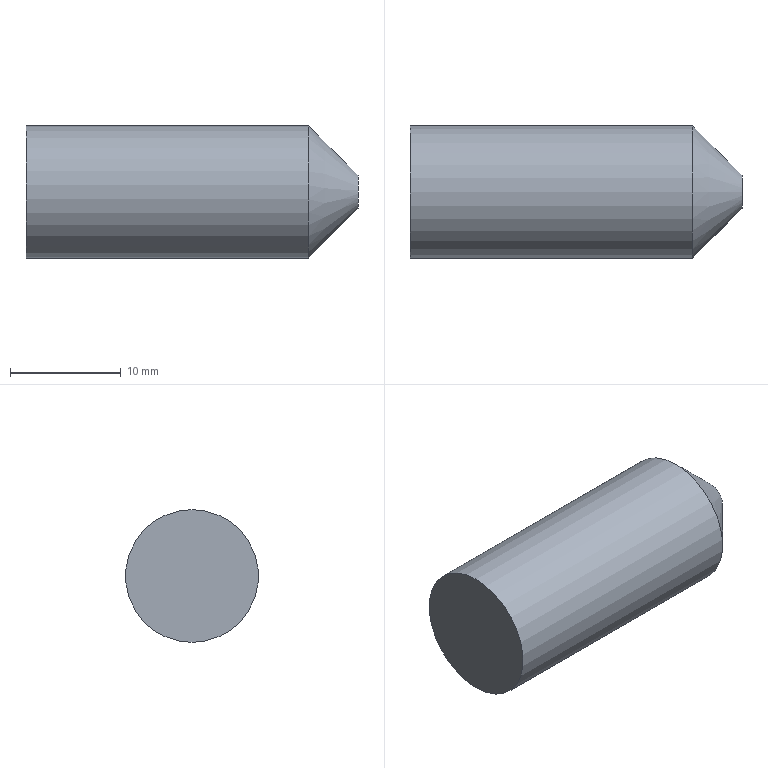Part | NX | features solid 2 | 1 solid | 4 faces | box 30 x 12 x 12 mm | volume 3107 mm3 | plane 2 | cylinder 1 | cone 1 | commonest cylinder face diameters 12 x1
STEP:
#1=CARTESIAN_POINT('',(-1510.,-494.26,-419.));
#2=VERTEX_POINT('',#1);
#3=CARTESIAN_POINT('',(-1510.,-494.26,-425.));
#4=DIRECTION('',(-1.,0.,0.));
#5=DIRECTION('',(0.,0.,1.));
#6=AXIS2_PLACEMENT_3D('',#3,#4,#5);
#7=CIRCLE('',#6,6.);
#8=EDGE_CURVE('',#2,#2,#7,.T.);
#9=ORIENTED_EDGE('',*,*,#8,.F.);
#10=EDGE_LOOP('',(#9));
#11=FACE_BOUND('',#10,.T.);
#12=CARTESIAN_POINT('',(-1484.5,-494.26,-419.));
#13=VERTEX_POINT('',#12);
#14=CARTESIAN_POINT('',(-1484.5,-494.26,-425.));
#15=DIRECTION('',(1.,0.,0.));
#16=DIRECTION('',(0.,0.,1.));
#17=AXIS2_PLACEMENT_3D('',#14,#15,#16);
#18=CIRCLE('',#17,6.);
#19=EDGE_CURVE('',#13,#13,#18,.F.);
#20=ORIENTED_EDGE('',*,*,#19,.T.);
#21=EDGE_LOOP('',(#20));
#22=FACE_BOUND('',#21,.T.);
#23=CARTESIAN_POINT('',(-1480.,-494.26,-425.));
#24=DIRECTION('',(-1.,0.,0.));
#25=DIRECTION('',(0.,0.,1.));
#26=AXIS2_PLACEMENT_3D('',#23,#24,#25);
#27=CYLINDRICAL_SURFACE('',#26,6.);
#28=ADVANCED_FACE('',(#11,#22),#27,.T.);
#29=ORIENTED_EDGE('',*,*,#8,.T.);
#30=EDGE_LOOP('',(#29));
#31=FACE_BOUND('',#30,.T.);
#32=CARTESIAN_POINT('',(-1510.,-494.26,-425.));
#33=DIRECTION('',(1.,0.,0.));
#34=DIRECTION('',(0.,0.,-1.));
#35=AXIS2_PLACEMENT_3D('',#32,#33,#34);
#36=PLANE('',#35);
#37=ADVANCED_FACE('',(#31),#36,.F.);
#38=CARTESIAN_POINT('',(-1480.,-494.26,-423.5));
#39=VERTEX_POINT('',#38);
#40=CARTESIAN_POINT('',(-1480.,-494.26,-425.));
#41=DIRECTION('',(-1.,0.,0.));
#42=DIRECTION('',(0.,0.,1.));
#43=AXIS2_PLACEMENT_3D('',#40,#41,#42);
#44=CIRCLE('',#43,1.5);
#45=EDGE_CURVE('',#39,#39,#44,.T.);
#46=ORIENTED_EDGE('',*,*,#45,.T.);
#47=EDGE_LOOP('',(#46));
#48=FACE_BOUND('',#47,.T.);
#49=ORIENTED_EDGE('',*,*,#19,.F.);
#50=EDGE_LOOP('',(#49));
#51=FACE_BOUND('',#50,.T.);
#52=CARTESIAN_POINT('',(-1480.,-494.26,-425.));
#53=DIRECTION('',(-1.,0.,0.));
#54=DIRECTION('',(0.,0.,1.));
#55=AXIS2_PLACEMENT_3D('',#52,#53,#54);
#56=CONICAL_SURFACE('',#55,1.5,0.7854);
#57=ADVANCED_FACE('',(#48,#51),#56,.T.);
#58=ORIENTED_EDGE('',*,*,#45,.F.);
#59=EDGE_LOOP('',(#58));
#60=FACE_BOUND('',#59,.T.);
#61=CARTESIAN_POINT('',(-1480.,-494.26,-425.));
#62=DIRECTION('',(1.,0.,0.));
#63=DIRECTION('',(0.,0.,-1.));
#64=AXIS2_PLACEMENT_3D('',#61,#62,#63);
#65=PLANE('',#64);
#66=ADVANCED_FACE('',(#60),#65,.T.);
#67=CLOSED_SHELL('',(#28,#37,#57,#66));
#68=MANIFOLD_SOLID_BREP('',#67);
#69=(LENGTH_UNIT()NAMED_UNIT(*)SI_UNIT(.MILLI.,.METRE.));
#70=UNCERTAINTY_MEASURE_WITH_UNIT(LENGTH_MEASURE(0.00001),#69,'','');
#71=(NAMED_UNIT(*)PLANE_ANGLE_UNIT()SI_UNIT($,.RADIAN.));
#72=(NAMED_UNIT(*)SI_UNIT($,.STERADIAN.)SOLID_ANGLE_UNIT());
#73=(GEOMETRIC_REPRESENTATION_CONTEXT(3)GLOBAL_UNCERTAINTY_ASSIGNED_CONTEXT((#70))GLOBAL_UNIT_ASSIGNED_CONTEXT((#69,#71,#72))REPRESENTATION_CONTEXT('',''));
#74=ADVANCED_BREP_SHAPE_REPRESENTATION('',(#68),#73);